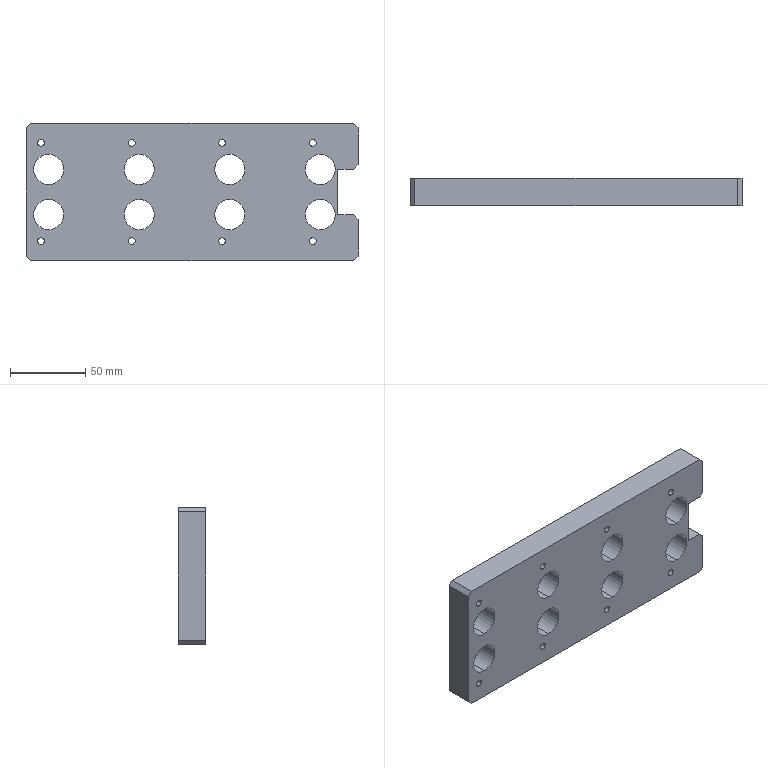Part | STEP file | 0-19 Battery pad plate | 1 solid | 72 faces | box 220 x 18 x 91 mm | volume 303845 mm3 | cylinder 48 | plane 24 | commonest cylinder face diameters 4.5 x16 8 x16 20 x16